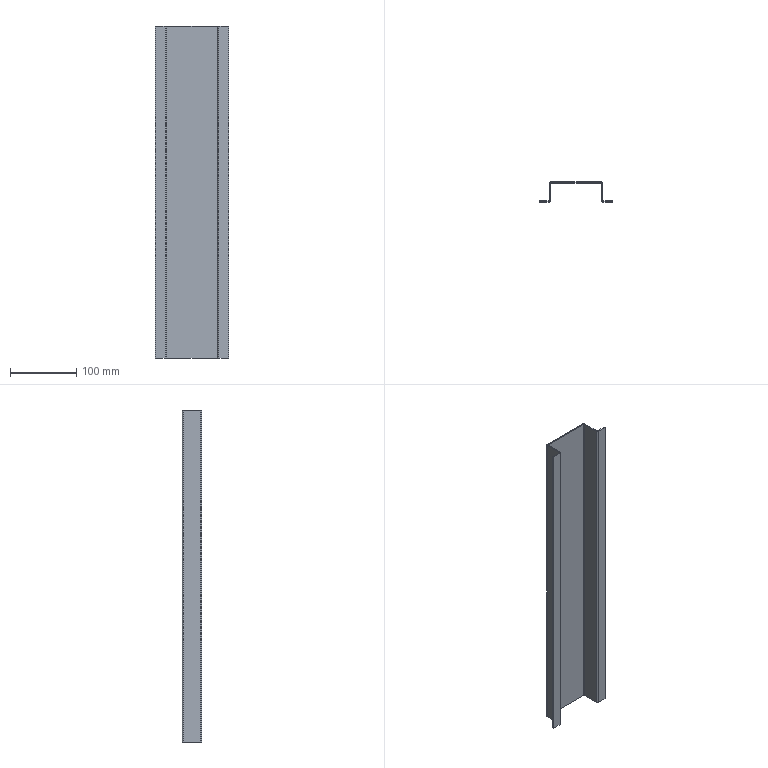Part | SolidWorks | features FlatPattern 1, SMBaseFlange 1, SheetMetal 1 | 1 solid | 38 faces | box 110 x 30 x 500 mm | volume 123640 mm3 | plane 30 | cylinder 8 | commonest cylinder face diameters 1 x4 4 x4
STEP:
#1=CARTESIAN_POINT('',(-40.,0.5,250.));
#2=VERTEX_POINT('',#1);
#3=CARTESIAN_POINT('',(-38.5,0.5,250.));
#4=VERTEX_POINT('',#3);
#5=CARTESIAN_POINT('',(-40.,0.5,250.));
#6=DIRECTION('',(1.,0.,0.));
#7=VECTOR('',#6,1000.);
#8=LINE('',#5,#7);
#9=EDGE_CURVE('',#2,#4,#8,.T.);
#10=ORIENTED_EDGE('',*,*,#9,.F.);
#11=CARTESIAN_POINT('',(-40.5,0.,250.));
#12=VERTEX_POINT('',#11);
#13=CARTESIAN_POINT('',(-40.5,0.5,250.));
#14=DIRECTION('',(0.,0.,-1.));
#15=DIRECTION('',(-1.,0.,0.));
#16=AXIS2_PLACEMENT_3D('',#13,#14,#15);
#17=CIRCLE('',#16,0.5);
#18=EDGE_CURVE('',#2,#12,#17,.T.);
#19=ORIENTED_EDGE('',*,*,#18,.T.);
#20=CARTESIAN_POINT('',(-40.5,-1.5,250.));
#21=VERTEX_POINT('',#20);
#22=CARTESIAN_POINT('',(-40.5,-1.5,250.));
#23=DIRECTION('',(0.,1.,0.));
#24=VECTOR('',#23,1000.);
#25=LINE('',#22,#24);
#26=EDGE_CURVE('',#21,#12,#25,.T.);
#27=ORIENTED_EDGE('',*,*,#26,.F.);
#28=CARTESIAN_POINT('',(-40.5,0.5,250.));
#29=DIRECTION('',(0.,0.,-1.));
#30=DIRECTION('',(1.,0.,0.));
#31=AXIS2_PLACEMENT_3D('',#28,#29,#30);
#32=CIRCLE('',#31,2.);
#33=EDGE_CURVE('',#4,#21,#32,.T.);
#34=ORIENTED_EDGE('',*,*,#33,.F.);
#35=EDGE_LOOP('',(#10,#19,#27,#34));
#36=FACE_OUTER_BOUND('',#35,.T.);
#37=CARTESIAN_POINT('',(-40.,0.5,250.));
#38=DIRECTION('',(0.,0.,1.));
#39=DIRECTION('',(1.,0.,0.));
#40=AXIS2_PLACEMENT_3D('',#37,#38,#39);
#41=PLANE('',#40);
#42=ADVANCED_FACE('',(#36),#41,.T.);
#43=CARTESIAN_POINT('',(-40.,26.5,250.));
#44=VERTEX_POINT('',#43);
#45=CARTESIAN_POINT('',(-40.,0.,250.));
#46=DIRECTION('',(0.,-1.,0.));
#47=VECTOR('',#46,1000.);
#48=LINE('',#45,#47);
#49=EDGE_CURVE('',#44,#2,#48,.T.);
#50=ORIENTED_EDGE('',*,*,#49,.T.);
#51=ORIENTED_EDGE('',*,*,#9,.T.);
#52=CARTESIAN_POINT('',(-38.5,26.5,250.));
#53=VERTEX_POINT('',#52);
#54=CARTESIAN_POINT('',(-38.5,0.,250.));
#55=DIRECTION('',(0.,-1.,0.));
#56=VECTOR('',#55,1000.);
#57=LINE('',#54,#56);
#58=EDGE_CURVE('',#53,#4,#57,.T.);
#59=ORIENTED_EDGE('',*,*,#58,.F.);
#60=CARTESIAN_POINT('',(-38.5,26.5,250.));
#61=DIRECTION('',(-1.,0.,0.));
#62=VECTOR('',#61,1000.);
#63=LINE('',#60,#62);
#64=EDGE_CURVE('',#53,#44,#63,.T.);
#65=ORIENTED_EDGE('',*,*,#64,.T.);
#66=EDGE_LOOP('',(#50,#51,#59,#65));
#67=FACE_OUTER_BOUND('',#66,.T.);
#68=CARTESIAN_POINT('',(-40.5,-1.5,250.));
#69=DIRECTION('',(0.,0.,1.));
#70=DIRECTION('',(1.,0.,0.));
#71=AXIS2_PLACEMENT_3D('',#68,#69,#70);
#72=PLANE('',#71);
#73=ADVANCED_FACE('',(#67),#72,.T.);
#74=CARTESIAN_POINT('',(-40.5,0.,-250.));
#75=VERTEX_POINT('',#74);
#76=CARTESIAN_POINT('',(-40.5,-1.5,-250.));
#77=VERTEX_POINT('',#76);
#78=CARTESIAN_POINT('',(-40.5,0.,-250.));
#79=DIRECTION('',(0.,-1.,0.));
#80=VECTOR('',#79,1000.);
#81=LINE('',#78,#80);
#82=EDGE_CURVE('',#75,#77,#81,.T.);
#83=ORIENTED_EDGE('',*,*,#82,.F.);
#84=CARTESIAN_POINT('',(-40.,0.5,-250.));
#85=VERTEX_POINT('',#84);
#86=CARTESIAN_POINT('',(-40.5,0.5,-250.));
#87=DIRECTION('',(0.,0.,-1.));
#88=DIRECTION('',(-1.,0.,0.));
#89=AXIS2_PLACEMENT_3D('',#86,#87,#88);
#90=CIRCLE('',#89,0.5);
#91=EDGE_CURVE('',#85,#75,#90,.T.);
#92=ORIENTED_EDGE('',*,*,#91,.F.);
#93=CARTESIAN_POINT('',(-38.5,0.5,-250.));
#94=VERTEX_POINT('',#93);
#95=CARTESIAN_POINT('',(-38.5,0.5,-250.));
#96=DIRECTION('',(-1.,0.,0.));
#97=VECTOR('',#96,1000.);
#98=LINE('',#95,#97);
#99=EDGE_CURVE('',#94,#85,#98,.T.);
#100=ORIENTED_EDGE('',*,*,#99,.F.);
#101=CARTESIAN_POINT('',(-40.5,0.5,-250.));
#102=DIRECTION('',(0.,0.,-1.));
#103=DIRECTION('',(1.,0.,0.));
#104=AXIS2_PLACEMENT_3D('',#101,#102,#103);
#105=CIRCLE('',#104,2.);
#106=EDGE_CURVE('',#94,#77,#105,.T.);
#107=ORIENTED_EDGE('',*,*,#106,.T.);
#108=EDGE_LOOP('',(#83,#92,#100,#107));
#109=FACE_OUTER_BOUND('',#108,.T.);
#110=CARTESIAN_POINT('',(-40.5,0.,-250.));
#111=DIRECTION('',(0.,0.,-1.));
#112=DIRECTION('',(-1.,0.,0.));
#113=AXIS2_PLACEMENT_3D('',#110,#111,#112);
#114=PLANE('',#113);
#115=ADVANCED_FACE('',(#109),#114,.T.);
#116=CARTESIAN_POINT('',(-55.,0.,-250.));
#117=VERTEX_POINT('',#116);
#118=CARTESIAN_POINT('',(-55.,0.,-250.));
#119=DIRECTION('',(-1.,0.,0.));
#120=VECTOR('',#119,1000.);
#121=LINE('',#118,#120);
#122=EDGE_CURVE('',#75,#117,#121,.T.);
#123=ORIENTED_EDGE('',*,*,#122,.F.);
#124=ORIENTED_EDGE('',*,*,#82,.T.);
#125=CARTESIAN_POINT('',(-55.,-1.5,-250.));
#126=VERTEX_POINT('',#125);
#127=CARTESIAN_POINT('',(-55.,-1.5,-250.));
#128=DIRECTION('',(-1.,0.,0.));
#129=VECTOR('',#128,1000.);
#130=LINE('',#127,#129);
#131=EDGE_CURVE('',#77,#126,#130,.T.);
#132=ORIENTED_EDGE('',*,*,#131,.T.);
#133=CARTESIAN_POINT('',(-55.,-1.5,-250.));
#134=DIRECTION('',(0.,1.,0.));
#135=VECTOR('',#134,1000.);
#136=LINE('',#133,#135);
#137=EDGE_CURVE('',#126,#117,#136,.T.);
#138=ORIENTED_EDGE('',*,*,#137,.T.);
#139=EDGE_LOOP('',(#123,#124,#132,#138));
#140=FACE_OUTER_BOUND('',#139,.T.);
#141=CARTESIAN_POINT('',(-38.5,0.5,-250.));
#142=DIRECTION('',(0.,0.,-1.));
#143=DIRECTION('',(-1.,0.,0.));
#144=AXIS2_PLACEMENT_3D('',#141,#142,#143);
#145=PLANE('',#144);
#146=ADVANCED_FACE('',(#140),#145,.T.);
#147=CARTESIAN_POINT('',(-38.,28.5,250.));
#148=VERTEX_POINT('',#147);
#149=CARTESIAN_POINT('',(-38.,27.,250.));
#150=VERTEX_POINT('',#149);
#151=CARTESIAN_POINT('',(-38.,28.5,250.));
#152=DIRECTION('',(0.,-1.,0.));
#153=VECTOR('',#152,1000.);
#154=LINE('',#151,#153);
#155=EDGE_CURVE('',#148,#150,#154,.T.);
#156=ORIENTED_EDGE('',*,*,#155,.F.);
#157=CARTESIAN_POINT('',(-38.,26.5,250.));
#158=DIRECTION('',(0.,0.,1.));
#159=DIRECTION('',(1.,0.,0.));
#160=AXIS2_PLACEMENT_3D('',#157,#158,#159);
#161=CIRCLE('',#160,2.);
#162=EDGE_CURVE('',#148,#44,#161,.T.);
#163=ORIENTED_EDGE('',*,*,#162,.T.);
#164=ORIENTED_EDGE('',*,*,#64,.F.);
#165=CARTESIAN_POINT('',(-38.,26.5,250.));
#166=DIRECTION('',(0.,0.,1.));
#167=DIRECTION('',(1.,0.,0.));
#168=AXIS2_PLACEMENT_3D('',#165,#166,#167);
#169=CIRCLE('',#168,0.5);
#170=EDGE_CURVE('',#150,#53,#169,.T.);
#171=ORIENTED_EDGE('',*,*,#170,.F.);
#172=EDGE_LOOP('',(#156,#163,#164,#171));
#173=FACE_OUTER_BOUND('',#172,.T.);
#174=CARTESIAN_POINT('',(-38.,28.5,250.));
#175=DIRECTION('',(0.,0.,1.));
#176=DIRECTION('',(1.,0.,0.));
#177=AXIS2_PLACEMENT_3D('',#174,#175,#176);
#178=PLANE('',#177);
#179=ADVANCED_FACE('',(#173),#178,.T.);
#180=CARTESIAN_POINT('',(38.,28.5,250.));
#181=VERTEX_POINT('',#180);
#182=CARTESIAN_POINT('',(-40.,28.5,250.));
#183=DIRECTION('',(-1.,0.,0.));
#184=VECTOR('',#183,1000.);
#185=LINE('',#182,#184);
#186=EDGE_CURVE('',#181,#148,#185,.T.);
#187=ORIENTED_EDGE('',*,*,#186,.T.);
#188=ORIENTED_EDGE('',*,*,#155,.T.);
#189=CARTESIAN_POINT('',(38.,27.,250.));
#190=VERTEX_POINT('',#189);
#191=CARTESIAN_POINT('',(-40.,27.,250.));
#192=DIRECTION('',(-1.,0.,0.));
#193=VECTOR('',#192,1000.);
#194=LINE('',#191,#193);
#195=EDGE_CURVE('',#190,#150,#194,.T.);
#196=ORIENTED_EDGE('',*,*,#195,.F.);
#197=CARTESIAN_POINT('',(38.,27.,250.));
#198=DIRECTION('',(0.,1.,0.));
#199=VECTOR('',#198,1000.);
#200=LINE('',#197,#199);
#201=EDGE_CURVE('',#190,#181,#200,.T.);
#202=ORIENTED_EDGE('',*,*,#201,.T.);
#203=EDGE_LOOP('',(#187,#188,#196,#202));
#204=FACE_OUTER_BOUND('',#203,.T.);
#205=CARTESIAN_POINT('',(-38.5,26.5,250.));
#206=DIRECTION('',(0.,0.,1.));
#207=DIRECTION('',(1.,0.,0.));
#208=AXIS2_PLACEMENT_3D('',#205,#206,#207);
#209=PLANE('',#208);
#210=ADVANCED_FACE('',(#204),#209,.T.);
#211=CARTESIAN_POINT('',(-40.,26.5,-250.));
#212=VERTEX_POINT('',#211);
#213=CARTESIAN_POINT('',(-38.5,26.5,-250.));
#214=VERTEX_POINT('',#213);
#215=CARTESIAN_POINT('',(-40.,26.5,-250.));
#216=DIRECTION('',(1.,0.,0.));
#217=VECTOR('',#216,1000.);
#218=LINE('',#215,#217);
#219=EDGE_CURVE('',#212,#214,#218,.T.);
#220=ORIENTED_EDGE('',*,*,#219,.F.);
#221=CARTESIAN_POINT('',(-38.,28.5,-250.));
#222=VERTEX_POINT('',#221);
#223=CARTESIAN_POINT('',(-38.,26.5,-250.));
#224=DIRECTION('',(0.,0.,1.));
#225=DIRECTION('',(1.,0.,0.));
#226=AXIS2_PLACEMENT_3D('',#223,#224,#225);
#227=CIRCLE('',#226,2.);
#228=EDGE_CURVE('',#222,#212,#227,.T.);
#229=ORIENTED_EDGE('',*,*,#228,.F.);
#230=CARTESIAN_POINT('',(-38.,27.,-250.));
#231=VERTEX_POINT('',#230);
#232=CARTESIAN_POINT('',(-38.,27.,-250.));
#233=DIRECTION('',(0.,1.,0.));
#234=VECTOR('',#233,1000.);
#235=LINE('',#232,#234);
#236=EDGE_CURVE('',#231,#222,#235,.T.);
#237=ORIENTED_EDGE('',*,*,#236,.F.);
#238=CARTESIAN_POINT('',(-38.,26.5,-250.));
#239=DIRECTION('',(0.,0.,1.));
#240=DIRECTION('',(1.,0.,0.));
#241=AXIS2_PLACEMENT_3D('',#238,#239,#240);
#242=CIRCLE('',#241,0.5);
#243=EDGE_CURVE('',#231,#214,#242,.T.);
#244=ORIENTED_EDGE('',*,*,#243,.T.);
#245=EDGE_LOOP('',(#220,#229,#237,#244));
#246=FACE_OUTER_BOUND('',#245,.T.);
#247=CARTESIAN_POINT('',(-40.,26.5,-250.));
#248=DIRECTION('',(0.,0.,-1.));
#249=DIRECTION('',(-1.,0.,0.));
#250=AXIS2_PLACEMENT_3D('',#247,#248,#249);
#251=PLANE('',#250);
#252=ADVANCED_FACE('',(#246),#251,.T.);
#253=CARTESIAN_POINT('',(-40.,0.,-250.));
#254=DIRECTION('',(0.,-1.,0.));
#255=VECTOR('',#254,1000.);
#256=LINE('',#253,#255);
#257=EDGE_CURVE('',#212,#85,#256,.T.);
#258=ORIENTED_EDGE('',*,*,#257,.F.);
#259=ORIENTED_EDGE('',*,*,#219,.T.);
#260=CARTESIAN_POINT('',(-38.5,0.,-250.));
#261=DIRECTION('',(0.,-1.,0.));
#262=VECTOR('',#261,1000.);
#263=LINE('',#260,#262);
#264=EDGE_CURVE('',#214,#94,#263,.T.);
#265=ORIENTED_EDGE('',*,*,#264,.T.);
#266=ORIENTED_EDGE('',*,*,#99,.T.);
#267=EDGE_LOOP('',(#258,#259,#265,#266));
#268=FACE_OUTER_BOUND('',#267,.T.);
#269=CARTESIAN_POINT('',(-38.,27.,-250.));
#270=DIRECTION('',(0.,0.,-1.));
#271=DIRECTION('',(-1.,0.,0.));
#272=AXIS2_PLACEMENT_3D('',#269,#270,#271);
#273=PLANE('',#272);
#274=ADVANCED_FACE('',(#268),#273,.T.);
#275=CARTESIAN_POINT('',(40.,26.5,250.));
#276=VERTEX_POINT('',#275);
#277=CARTESIAN_POINT('',(38.5,26.5,250.));
#278=VERTEX_POINT('',#277);
#279=CARTESIAN_POINT('',(40.,26.5,250.));
#280=DIRECTION('',(-1.,0.,0.));
#281=VECTOR('',#280,1000.);
#282=LINE('',#279,#281);
#283=EDGE_CURVE('',#276,#278,#282,.T.);
#284=ORIENTED_EDGE('',*,*,#283,.F.);
#285=CARTESIAN_POINT('',(38.,26.5,250.));
#286=DIRECTION('',(0.,0.,1.));
#287=DIRECTION('',(1.,0.,0.));
#288=AXIS2_PLACEMENT_3D('',#285,#286,#287);
#289=CIRCLE('',#288,2.);
#290=EDGE_CURVE('',#276,#181,#289,.T.);
#291=ORIENTED_EDGE('',*,*,#290,.T.);
#292=ORIENTED_EDGE('',*,*,#201,.F.);
#293=CARTESIAN_POINT('',(38.,26.5,250.));
#294=DIRECTION('',(0.,0.,1.));
#295=DIRECTION('',(1.,0.,0.));
#296=AXIS2_PLACEMENT_3D('',#293,#294,#295);
#297=CIRCLE('',#296,0.5);
#298=EDGE_CURVE('',#278,#190,#297,.T.);
#299=ORIENTED_EDGE('',*,*,#298,.F.);
#300=EDGE_LOOP('',(#284,#291,#292,#299));
#301=FACE_OUTER_BOUND('',#300,.T.);
#302=CARTESIAN_POINT('',(40.,26.5,250.));
#303=DIRECTION('',(0.,0.,1.));
#304=DIRECTION('',(1.,0.,0.));
#305=AXIS2_PLACEMENT_3D('',#302,#303,#304);
#306=PLANE('',#305);
#307=ADVANCED_FACE('',(#301),#306,.T.);
#308=CARTESIAN_POINT('',(40.,0.5,250.));
#309=VERTEX_POINT('',#308);
#310=CARTESIAN_POINT('',(40.,0.,250.));
#311=DIRECTION('',(0.,1.,0.));
#312=VECTOR('',#311,1000.);
#313=LINE('',#310,#312);
#314=EDGE_CURVE('',#309,#276,#313,.T.);
#315=ORIENTED_EDGE('',*,*,#314,.T.);
#316=ORIENTED_EDGE('',*,*,#283,.T.);
#317=CARTESIAN_POINT('',(38.5,0.5,250.));
#318=VERTEX_POINT('',#317);
#319=CARTESIAN_POINT('',(38.5,0.,250.));
#320=DIRECTION('',(0.,1.,0.));
#321=VECTOR('',#320,1000.);
#322=LINE('',#319,#321);
#323=EDGE_CURVE('',#318,#278,#322,.T.);
#324=ORIENTED_EDGE('',*,*,#323,.F.);
#325=CARTESIAN_POINT('',(38.5,0.5,250.));
#326=DIRECTION('',(1.,0.,0.));
#327=VECTOR('',#326,1000.);
#328=LINE('',#325,#327);
#329=EDGE_CURVE('',#318,#309,#328,.T.);
#330=ORIENTED_EDGE('',*,*,#329,.T.);
#331=EDGE_LOOP('',(#315,#316,#324,#330));
#332=FACE_OUTER_BOUND('',#331,.T.);
#333=CARTESIAN_POINT('',(38.,27.,250.));
#334=DIRECTION('',(0.,0.,1.));
#335=DIRECTION('',(1.,0.,0.));
#336=AXIS2_PLACEMENT_3D('',#333,#334,#335);
#337=PLANE('',#336);
#338=ADVANCED_FACE('',(#332),#337,.T.);
#339=CARTESIAN_POINT('',(38.,28.5,-250.));
#340=VERTEX_POINT('',#339);
#341=CARTESIAN_POINT('',(38.,27.,-250.));
#342=VERTEX_POINT('',#341);
#343=CARTESIAN_POINT('',(38.,28.5,-250.));
#344=DIRECTION('',(0.,-1.,0.));
#345=VECTOR('',#344,1000.);
#346=LINE('',#343,#345);
#347=EDGE_CURVE('',#340,#342,#346,.T.);
#348=ORIENTED_EDGE('',*,*,#347,.F.);
#349=CARTESIAN_POINT('',(40.,26.5,-250.));
#350=VERTEX_POINT('',#349);
#351=CARTESIAN_POINT('',(38.,26.5,-250.));
#352=DIRECTION('',(0.,0.,1.));
#353=DIRECTION('',(1.,0.,0.));
#354=AXIS2_PLACEMENT_3D('',#351,#352,#353);
#355=CIRCLE('',#354,2.);
#356=EDGE_CURVE('',#350,#340,#355,.T.);
#357=ORIENTED_EDGE('',*,*,#356,.F.);
#358=CARTESIAN_POINT('',(38.5,26.5,-250.));
#359=VERTEX_POINT('',#358);
#360=CARTESIAN_POINT('',(38.5,26.5,-250.));
#361=DIRECTION('',(1.,0.,0.));
#362=VECTOR('',#361,1000.);
#363=LINE('',#360,#362);
#364=EDGE_CURVE('',#359,#350,#363,.T.);
#365=ORIENTED_EDGE('',*,*,#364,.F.);
#366=CARTESIAN_POINT('',(38.,26.5,-250.));
#367=DIRECTION('',(0.,0.,1.));
#368=DIRECTION('',(1.,0.,0.));
#369=AXIS2_PLACEMENT_3D('',#366,#367,#368);
#370=CIRCLE('',#369,0.5);
#371=EDGE_CURVE('',#359,#342,#370,.T.);
#372=ORIENTED_EDGE('',*,*,#371,.T.);
#373=EDGE_LOOP('',(#348,#357,#365,#372));
#374=FACE_OUTER_BOUND('',#373,.T.);
#375=CARTESIAN_POINT('',(38.,28.5,-250.));
#376=DIRECTION('',(0.,0.,-1.));
#377=DIRECTION('',(-1.,0.,0.));
#378=AXIS2_PLACEMENT_3D('',#375,#376,#377);
#379=PLANE('',#378);
#380=ADVANCED_FACE('',(#374),#379,.T.);
#381=CARTESIAN_POINT('',(-40.,28.5,-250.));
#382=DIRECTION('',(-1.,0.,0.));
#383=VECTOR('',#382,1000.);
#384=LINE('',#381,#383);
#385=EDGE_CURVE('',#340,#222,#384,.T.);
#386=ORIENTED_EDGE('',*,*,#385,.F.);
#387=ORIENTED_EDGE('',*,*,#347,.T.);
#388=CARTESIAN_POINT('',(-40.,27.,-250.));
#389=DIRECTION('',(-1.,0.,0.));
#390=VECTOR('',#389,1000.);
#391=LINE('',#388,#390);
#392=EDGE_CURVE('',#342,#231,#391,.T.);
#393=ORIENTED_EDGE('',*,*,#392,.T.);
#394=ORIENTED_EDGE('',*,*,#236,.T.);
#395=EDGE_LOOP('',(#386,#387,#393,#394));
#396=FACE_OUTER_BOUND('',#395,.T.);
#397=CARTESIAN_POINT('',(38.5,26.5,-250.));
#398=DIRECTION('',(0.,0.,-1.));
#399=DIRECTION('',(-1.,0.,0.));
#400=AXIS2_PLACEMENT_3D('',#397,#398,#399);
#401=PLANE('',#400);
#402=ADVANCED_FACE('',(#396),#401,.T.);
#403=CARTESIAN_POINT('',(40.5,0.,250.));
#404=VERTEX_POINT('',#403);
#405=CARTESIAN_POINT('',(40.5,-1.5,250.));
#406=VERTEX_POINT('',#405);
#407=CARTESIAN_POINT('',(40.5,0.,250.));
#408=DIRECTION('',(0.,-1.,0.));
#409=VECTOR('',#408,1000.);
#410=LINE('',#407,#409);
#411=EDGE_CURVE('',#404,#406,#410,.T.);
#412=ORIENTED_EDGE('',*,*,#411,.F.);
#413=CARTESIAN_POINT('',(40.5,0.5,250.));
#414=DIRECTION('',(0.,0.,-1.));
#415=DIRECTION('',(-1.,0.,0.));
#416=AXIS2_PLACEMENT_3D('',#413,#414,#415);
#417=CIRCLE('',#416,0.5);
#418=EDGE_CURVE('',#404,#309,#417,.T.);
#419=ORIENTED_EDGE('',*,*,#418,.T.);
#420=ORIENTED_EDGE('',*,*,#329,.F.);
#421=CARTESIAN_POINT('',(40.5,0.5,250.));
#422=DIRECTION('',(0.,0.,-1.));
#423=DIRECTION('',(1.,0.,0.));
#424=AXIS2_PLACEMENT_3D('',#421,#422,#423);
#425=CIRCLE('',#424,2.);
#426=EDGE_CURVE('',#406,#318,#425,.T.);
#427=ORIENTED_EDGE('',*,*,#426,.F.);
#428=EDGE_LOOP('',(#412,#419,#420,#427));
#429=FACE_OUTER_BOUND('',#428,.T.);
#430=CARTESIAN_POINT('',(40.5,0.,250.));
#431=DIRECTION('',(0.,0.,1.));
#432=DIRECTION('',(1.,0.,0.));
#433=AXIS2_PLACEMENT_3D('',#430,#431,#432);
#434=PLANE('',#433);
#435=ADVANCED_FACE('',(#429),#434,.T.);
#436=CARTESIAN_POINT('',(55.,0.,250.));
#437=VERTEX_POINT('',#436);
#438=CARTESIAN_POINT('',(55.,0.,250.));
#439=DIRECTION('',(-1.,0.,0.));
#440=VECTOR('',#439,1000.);
#441=LINE('',#438,#440);
#442=EDGE_CURVE('',#437,#404,#441,.T.);
#443=ORIENTED_EDGE('',*,*,#442,.T.);
#444=ORIENTED_EDGE('',*,*,#411,.T.);
#445=CARTESIAN_POINT('',(55.,-1.5,250.));
#446=VERTEX_POINT('',#445);
#447=CARTESIAN_POINT('',(55.,-1.5,250.));
#448=DIRECTION('',(-1.,0.,0.));
#449=VECTOR('',#448,1000.);
#450=LINE('',#447,#449);
#451=EDGE_CURVE('',#446,#406,#450,.T.);
#452=ORIENTED_EDGE('',*,*,#451,.F.);
#453=CARTESIAN_POINT('',(55.,0.,250.));
#454=DIRECTION('',(0.,-1.,0.));
#455=VECTOR('',#454,1000.);
#456=LINE('',#453,#455);
#457=EDGE_CURVE('',#437,#446,#456,.T.);
#458=ORIENTED_EDGE('',*,*,#457,.F.);
#459=EDGE_LOOP('',(#443,#444,#452,#458));
#460=FACE_OUTER_BOUND('',#459,.T.);
#461=CARTESIAN_POINT('',(38.5,0.5,250.));
#462=DIRECTION('',(0.,0.,1.));
#463=DIRECTION('',(1.,0.,0.));
#464=AXIS2_PLACEMENT_3D('',#461,#462,#463);
#465=PLANE('',#464);
#466=ADVANCED_FACE('',(#460),#465,.T.);
#467=CARTESIAN_POINT('',(40.,0.5,-250.));
#468=VERTEX_POINT('',#467);
#469=CARTESIAN_POINT('',(38.5,0.5,-250.));
#470=VERTEX_POINT('',#469);
#471=CARTESIAN_POINT('',(40.,0.5,-250.));
#472=DIRECTION('',(-1.,0.,0.));
#473=VECTOR('',#472,1000.);
#474=LINE('',#471,#473);
#475=EDGE_CURVE('',#468,#470,#474,.T.);
#476=ORIENTED_EDGE('',*,*,#475,.F.);
#477=CARTESIAN_POINT('',(40.5,0.,-250.));
#478=VERTEX_POINT('',#477);
#479=CARTESIAN_POINT('',(40.5,0.5,-250.));
#480=DIRECTION('',(0.,0.,-1.));
#481=DIRECTION('',(-1.,0.,0.));
#482=AXIS2_PLACEMENT_3D('',#479,#480,#481);
#483=CIRCLE('',#482,0.5);
#484=EDGE_CURVE('',#478,#468,#483,.T.);
#485=ORIENTED_EDGE('',*,*,#484,.F.);
#486=CARTESIAN_POINT('',(40.5,-1.5,-250.));
#487=VERTEX_POINT('',#486);
#488=CARTESIAN_POINT('',(40.5,-1.5,-250.));
#489=DIRECTION('',(0.,1.,0.));
#490=VECTOR('',#489,1000.);
#491=LINE('',#488,#490);
#492=EDGE_CURVE('',#487,#478,#491,.T.);
#493=ORIENTED_EDGE('',*,*,#492,.F.);
#494=CARTESIAN_POINT('',(40.5,0.5,-250.));
#495=DIRECTION('',(0.,0.,-1.));
#496=DIRECTION('',(1.,0.,0.));
#497=AXIS2_PLACEMENT_3D('',#494,#495,#496);
#498=CIRCLE('',#497,2.);
#499=EDGE_CURVE('',#487,#470,#498,.T.);
#500=ORIENTED_EDGE('',*,*,#499,.T.);
#501=EDGE_LOOP('',(#476,#485,#493,#500));
#502=FACE_OUTER_BOUND('',#501,.T.);
#503=CARTESIAN_POINT('',(40.,0.5,-250.));
#504=DIRECTION('',(0.,0.,-1.));
#505=DIRECTION('',(-1.,0.,0.));
#506=AXIS2_PLACEMENT_3D('',#503,#504,#505);
#507=PLANE('',#506);
#508=ADVANCED_FACE('',(#502),#507,.T.);
#509=CARTESIAN_POINT('',(40.,0.,-250.));
#510=DIRECTION('',(0.,1.,0.));
#511=VECTOR('',#510,1000.);
#512=LINE('',#509,#511);
#513=EDGE_CURVE('',#468,#350,#512,.T.);
#514=ORIENTED_EDGE('',*,*,#513,.F.);
#515=ORIENTED_EDGE('',*,*,#475,.T.);
#516=CARTESIAN_POINT('',(38.5,0.,-250.));
#517=DIRECTION('',(0.,1.,0.));
#518=VECTOR('',#517,1000.);
#519=LINE('',#516,#518);
#520=EDGE_CURVE('',#470,#359,#519,.T.);
#521=ORIENTED_EDGE('',*,*,#520,.T.);
#522=ORIENTED_EDGE('',*,*,#364,.T.);
#523=EDGE_LOOP('',(#514,#515,#521,#522));
#524=FACE_OUTER_BOUND('',#523,.T.);
#525=CARTESIAN_POINT('',(40.5,-1.5,-250.));
#526=DIRECTION('',(0.,0.,-1.));
#527=DIRECTION('',(-1.,0.,0.));
#528=AXIS2_PLACEMENT_3D('',#525,#526,#527);
#529=PLANE('',#528);
#530=ADVANCED_FACE('',(#524),#529,.T.);
#531=ORIENTED_EDGE('',*,*,#122,.T.);
#532=CARTESIAN_POINT('',(-55.,0.,250.));
#533=VERTEX_POINT('',#532);
#534=CARTESIAN_POINT('',(-55.,0.,250.));
#535=DIRECTION('',(0.,0.,-1.));
#536=VECTOR('',#535,1000.);
#537=LINE('',#534,#536);
#538=EDGE_CURVE('',#533,#117,#537,.T.);
#539=ORIENTED_EDGE('',*,*,#538,.F.);
#540=CARTESIAN_POINT('',(-55.,0.,250.));
#541=DIRECTION('',(-1.,0.,0.));
#542=VECTOR('',#541,1000.);
#543=LINE('',#540,#542);
#544=EDGE_CURVE('',#12,#533,#543,.T.);
#545=ORIENTED_EDGE('',*,*,#544,.F.);
#546=CARTESIAN_POINT('',(-40.5,0.,250.));
#547=DIRECTION('',(0.,0.,-1.));
#548=VECTOR('',#547,1000.);
#549=LINE('',#546,#548);
#550=EDGE_CURVE('',#12,#75,#549,.T.);
#551=ORIENTED_EDGE('',*,*,#550,.T.);
#552=EDGE_LOOP('',(#531,#539,#545,#551));
#553=FACE_OUTER_BOUND('',#552,.T.);
#554=CARTESIAN_POINT('',(-55.,0.,250.));
#555=DIRECTION('',(0.,-1.,0.));
#556=DIRECTION('',(0.,0.,-1.));
#557=AXIS2_PLACEMENT_3D('',#554,#555,#556);
#558=PLANE('',#557);
#559=ADVANCED_FACE('',(#553),#558,.F.);
#560=ORIENTED_EDGE('',*,*,#137,.F.);
#561=CARTESIAN_POINT('',(-55.,-1.5,250.));
#562=VERTEX_POINT('',#561);
#563=CARTESIAN_POINT('',(-55.,-1.5,250.));
#564=DIRECTION('',(0.,0.,-1.));
#565=VECTOR('',#564,1000.);
#566=LINE('',#563,#565);
#567=EDGE_CURVE('',#562,#126,#566,.T.);
#568=ORIENTED_EDGE('',*,*,#567,.F.);
#569=CARTESIAN_POINT('',(-55.,-1.5,250.));
#570=DIRECTION('',(0.,1.,0.));
#571=VECTOR('',#570,1000.);
#572=LINE('',#569,#571);
#573=EDGE_CURVE('',#562,#533,#572,.T.);
#574=ORIENTED_EDGE('',*,*,#573,.T.);
#575=ORIENTED_EDGE('',*,*,#538,.T.);
#576=EDGE_LOOP('',(#560,#568,#574,#575));
#577=FACE_OUTER_BOUND('',#576,.T.);
#578=CARTESIAN_POINT('',(-55.,-1.5,250.));
#579=DIRECTION('',(-1.,0.,0.));
#580=DIRECTION('',(0.,0.,1.));
#581=AXIS2_PLACEMENT_3D('',#578,#579,#580);
#582=PLANE('',#581);
#583=ADVANCED_FACE('',(#577),#582,.T.);
#584=ORIENTED_EDGE('',*,*,#131,.F.);
#585=CARTESIAN_POINT('',(-40.5,-1.5,250.));
#586=DIRECTION('',(0.,0.,-1.));
#587=VECTOR('',#586,1000.);
#588=LINE('',#585,#587);
#589=EDGE_CURVE('',#21,#77,#588,.T.);
#590=ORIENTED_EDGE('',*,*,#589,.F.);
#591=CARTESIAN_POINT('',(-55.,-1.5,250.));
#592=DIRECTION('',(-1.,0.,0.));
#593=VECTOR('',#592,1000.);
#594=LINE('',#591,#593);
#595=EDGE_CURVE('',#21,#562,#594,.T.);
#596=ORIENTED_EDGE('',*,*,#595,.T.);
#597=ORIENTED_EDGE('',*,*,#567,.T.);
#598=EDGE_LOOP('',(#584,#590,#596,#597));
#599=FACE_OUTER_BOUND('',#598,.T.);
#600=CARTESIAN_POINT('',(-55.,-1.5,250.));
#601=DIRECTION('',(0.,-1.,0.));
#602=DIRECTION('',(0.,0.,-1.));
#603=AXIS2_PLACEMENT_3D('',#600,#601,#602);
#604=PLANE('',#603);
#605=ADVANCED_FACE('',(#599),#604,.T.);
#606=ORIENTED_EDGE('',*,*,#106,.F.);
#607=CARTESIAN_POINT('',(-38.5,0.5,250.));
#608=DIRECTION('',(0.,0.,-1.));
#609=VECTOR('',#608,1000.);
#610=LINE('',#607,#609);
#611=EDGE_CURVE('',#4,#94,#610,.T.);
#612=ORIENTED_EDGE('',*,*,#611,.F.);
#613=ORIENTED_EDGE('',*,*,#33,.T.);
#614=ORIENTED_EDGE('',*,*,#589,.T.);
#615=EDGE_LOOP('',(#606,#612,#613,#614));
#616=FACE_OUTER_BOUND('',#615,.T.);
#617=CARTESIAN_POINT('',(-40.5,0.5,250.));
#618=DIRECTION('',(0.,0.,-1.));
#619=DIRECTION('',(-1.,0.,0.));
#620=AXIS2_PLACEMENT_3D('',#617,#618,#619);
#621=CYLINDRICAL_SURFACE('',#620,2.);
#622=ADVANCED_FACE('',(#616),#621,.T.);
#623=ORIENTED_EDGE('',*,*,#264,.F.);
#624=CARTESIAN_POINT('',(-38.5,26.5,250.));
#625=DIRECTION('',(0.,0.,-1.));
#626=VECTOR('',#625,1000.);
#627=LINE('',#624,#626);
#628=EDGE_CURVE('',#53,#214,#627,.T.);
#629=ORIENTED_EDGE('',*,*,#628,.F.);
#630=ORIENTED_EDGE('',*,*,#58,.T.);
#631=ORIENTED_EDGE('',*,*,#611,.T.);
#632=EDGE_LOOP('',(#623,#629,#630,#631));
#633=FACE_OUTER_BOUND('',#632,.T.);
#634=CARTESIAN_POINT('',(-38.5,0.,250.));
#635=DIRECTION('',(1.,0.,0.));
#636=DIRECTION('',(0.,1.,0.));
#637=AXIS2_PLACEMENT_3D('',#634,#635,#636);
#638=PLANE('',#637);
#639=ADVANCED_FACE('',(#633),#638,.T.);
#640=ORIENTED_EDGE('',*,*,#243,.F.);
#641=CARTESIAN_POINT('',(-38.,27.,250.));
#642=DIRECTION('',(0.,0.,-1.));
#643=VECTOR('',#642,1000.);
#644=LINE('',#641,#643);
#645=EDGE_CURVE('',#150,#231,#644,.T.);
#646=ORIENTED_EDGE('',*,*,#645,.F.);
#647=ORIENTED_EDGE('',*,*,#170,.T.);
#648=ORIENTED_EDGE('',*,*,#628,.T.);
#649=EDGE_LOOP('',(#640,#646,#647,#648));
#650=FACE_OUTER_BOUND('',#649,.T.);
#651=CARTESIAN_POINT('',(-38.,26.5,250.));
#652=DIRECTION('',(0.,0.,-1.));
#653=DIRECTION('',(-1.,0.,0.));
#654=AXIS2_PLACEMENT_3D('',#651,#652,#653);
#655=CYLINDRICAL_SURFACE('',#654,0.5);
#656=ADVANCED_FACE('',(#650),#655,.F.);
#657=ORIENTED_EDGE('',*,*,#392,.F.);
#658=CARTESIAN_POINT('',(38.,27.,250.));
#659=DIRECTION('',(0.,0.,-1.));
#660=VECTOR('',#659,1000.);
#661=LINE('',#658,#660);
#662=EDGE_CURVE('',#190,#342,#661,.T.);
#663=ORIENTED_EDGE('',*,*,#662,.F.);
#664=ORIENTED_EDGE('',*,*,#195,.T.);
#665=ORIENTED_EDGE('',*,*,#645,.T.);
#666=EDGE_LOOP('',(#657,#663,#664,#665));
#667=FACE_OUTER_BOUND('',#666,.T.);
#668=CARTESIAN_POINT('',(-40.,27.,250.));
#669=DIRECTION('',(0.,-1.,0.));
#670=DIRECTION('',(0.,0.,-1.));
#671=AXIS2_PLACEMENT_3D('',#668,#669,#670);
#672=PLANE('',#671);
#673=ADVANCED_FACE('',(#667),#672,.T.);
#674=ORIENTED_EDGE('',*,*,#371,.F.);
#675=CARTESIAN_POINT('',(38.5,26.5,250.));
#676=DIRECTION('',(0.,0.,-1.));
#677=VECTOR('',#676,1000.);
#678=LINE('',#675,#677);
#679=EDGE_CURVE('',#278,#359,#678,.T.);
#680=ORIENTED_EDGE('',*,*,#679,.F.);
#681=ORIENTED_EDGE('',*,*,#298,.T.);
#682=ORIENTED_EDGE('',*,*,#662,.T.);
#683=EDGE_LOOP('',(#674,#680,#681,#682));
#684=FACE_OUTER_BOUND('',#683,.T.);
#685=CARTESIAN_POINT('',(38.,26.5,250.));
#686=DIRECTION('',(0.,0.,-1.));
#687=DIRECTION('',(-1.,0.,0.));
#688=AXIS2_PLACEMENT_3D('',#685,#686,#687);
#689=CYLINDRICAL_SURFACE('',#688,0.5);
#690=ADVANCED_FACE('',(#684),#689,.F.);
#691=ORIENTED_EDGE('',*,*,#520,.F.);
#692=CARTESIAN_POINT('',(38.5,0.5,250.));
#693=DIRECTION('',(0.,0.,-1.));
#694=VECTOR('',#693,1000.);
#695=LINE('',#692,#694);
#696=EDGE_CURVE('',#318,#470,#695,.T.);
#697=ORIENTED_EDGE('',*,*,#696,.F.);
#698=ORIENTED_EDGE('',*,*,#323,.T.);
#699=ORIENTED_EDGE('',*,*,#679,.T.);
#700=EDGE_LOOP('',(#691,#697,#698,#699));
#701=FACE_OUTER_BOUND('',#700,.T.);
#702=CARTESIAN_POINT('',(38.5,0.,250.));
#703=DIRECTION('',(-1.,0.,0.));
#704=DIRECTION('',(0.,-1.,0.));
#705=AXIS2_PLACEMENT_3D('',#702,#703,#704);
#706=PLANE('',#705);
#707=ADVANCED_FACE('',(#701),#706,.T.);
#708=ORIENTED_EDGE('',*,*,#499,.F.);
#709=CARTESIAN_POINT('',(40.5,-1.5,250.));
#710=DIRECTION('',(0.,0.,-1.));
#711=VECTOR('',#710,1000.);
#712=LINE('',#709,#711);
#713=EDGE_CURVE('',#406,#487,#712,.T.);
#714=ORIENTED_EDGE('',*,*,#713,.F.);
#715=ORIENTED_EDGE('',*,*,#426,.T.);
#716=ORIENTED_EDGE('',*,*,#696,.T.);
#717=EDGE_LOOP('',(#708,#714,#715,#716));
#718=FACE_OUTER_BOUND('',#717,.T.);
#719=CARTESIAN_POINT('',(40.5,0.5,250.));
#720=DIRECTION('',(0.,0.,-1.));
#721=DIRECTION('',(-1.,0.,0.));
#722=AXIS2_PLACEMENT_3D('',#719,#720,#721);
#723=CYLINDRICAL_SURFACE('',#722,2.);
#724=ADVANCED_FACE('',(#718),#723,.T.);
#725=CARTESIAN_POINT('',(55.,-1.5,-250.));
#726=VERTEX_POINT('',#725);
#727=CARTESIAN_POINT('',(55.,-1.5,-250.));
#728=DIRECTION('',(-1.,0.,0.));
#729=VECTOR('',#728,1000.);
#730=LINE('',#727,#729);
#731=EDGE_CURVE('',#726,#487,#730,.T.);
#732=ORIENTED_EDGE('',*,*,#731,.F.);
#733=CARTESIAN_POINT('',(55.,-1.5,250.));
#734=DIRECTION('',(0.,0.,-1.));
#735=VECTOR('',#734,1000.);
#736=LINE('',#733,#735);
#737=EDGE_CURVE('',#446,#726,#736,.T.);
#738=ORIENTED_EDGE('',*,*,#737,.F.);
#739=ORIENTED_EDGE('',*,*,#451,.T.);
#740=ORIENTED_EDGE('',*,*,#713,.T.);
#741=EDGE_LOOP('',(#732,#738,#739,#740));
#742=FACE_OUTER_BOUND('',#741,.T.);
#743=CARTESIAN_POINT('',(55.,-1.5,250.));
#744=DIRECTION('',(0.,-1.,0.));
#745=DIRECTION('',(0.,0.,-1.));
#746=AXIS2_PLACEMENT_3D('',#743,#744,#745);
#747=PLANE('',#746);
#748=ADVANCED_FACE('',(#742),#747,.T.);
#749=CARTESIAN_POINT('',(55.,0.,-250.));
#750=VERTEX_POINT('',#749);
#751=CARTESIAN_POINT('',(55.,0.,-250.));
#752=DIRECTION('',(0.,-1.,0.));
#753=VECTOR('',#752,1000.);
#754=LINE('',#751,#753);
#755=EDGE_CURVE('',#750,#726,#754,.T.);
#756=ORIENTED_EDGE('',*,*,#755,.F.);
#757=CARTESIAN_POINT('',(55.,0.,250.));
#758=DIRECTION('',(0.,0.,-1.));
#759=VECTOR('',#758,1000.);
#760=LINE('',#757,#759);
#761=EDGE_CURVE('',#437,#750,#760,.T.);
#762=ORIENTED_EDGE('',*,*,#761,.F.);
#763=ORIENTED_EDGE('',*,*,#457,.T.);
#764=ORIENTED_EDGE('',*,*,#737,.T.);
#765=EDGE_LOOP('',(#756,#762,#763,#764));
#766=FACE_OUTER_BOUND('',#765,.T.);
#767=CARTESIAN_POINT('',(55.,0.,250.));
#768=DIRECTION('',(1.,0.,0.));
#769=DIRECTION('',(0.,0.,-1.));
#770=AXIS2_PLACEMENT_3D('',#767,#768,#769);
#771=PLANE('',#770);
#772=ADVANCED_FACE('',(#766),#771,.T.);
#773=CARTESIAN_POINT('',(55.,0.,-250.));
#774=DIRECTION('',(-1.,0.,0.));
#775=VECTOR('',#774,1000.);
#776=LINE('',#773,#775);
#777=EDGE_CURVE('',#750,#478,#776,.T.);
#778=ORIENTED_EDGE('',*,*,#777,.T.);
#779=CARTESIAN_POINT('',(40.5,0.,250.));
#780=DIRECTION('',(0.,0.,-1.));
#781=VECTOR('',#780,1000.);
#782=LINE('',#779,#781);
#783=EDGE_CURVE('',#404,#478,#782,.T.);
#784=ORIENTED_EDGE('',*,*,#783,.F.);
#785=ORIENTED_EDGE('',*,*,#442,.F.);
#786=ORIENTED_EDGE('',*,*,#761,.T.);
#787=EDGE_LOOP('',(#778,#784,#785,#786));
#788=FACE_OUTER_BOUND('',#787,.T.);
#789=CARTESIAN_POINT('',(55.,0.,250.));
#790=DIRECTION('',(0.,-1.,0.));
#791=DIRECTION('',(0.,0.,-1.));
#792=AXIS2_PLACEMENT_3D('',#789,#790,#791);
#793=PLANE('',#792);
#794=ADVANCED_FACE('',(#788),#793,.F.);
#795=ORIENTED_EDGE('',*,*,#484,.T.);
#796=CARTESIAN_POINT('',(40.,0.5,250.));
#797=DIRECTION('',(0.,0.,-1.));
#798=VECTOR('',#797,1000.);
#799=LINE('',#796,#798);
#800=EDGE_CURVE('',#309,#468,#799,.T.);
#801=ORIENTED_EDGE('',*,*,#800,.F.);
#802=ORIENTED_EDGE('',*,*,#418,.F.);
#803=ORIENTED_EDGE('',*,*,#783,.T.);
#804=EDGE_LOOP('',(#795,#801,#802,#803));
#805=FACE_OUTER_BOUND('',#804,.T.);
#806=CARTESIAN_POINT('',(40.5,0.5,250.));
#807=DIRECTION('',(0.,0.,-1.));
#808=DIRECTION('',(-1.,0.,0.));
#809=AXIS2_PLACEMENT_3D('',#806,#807,#808);
#810=CYLINDRICAL_SURFACE('',#809,0.5);
#811=ADVANCED_FACE('',(#805),#810,.F.);
#812=ORIENTED_EDGE('',*,*,#513,.T.);
#813=CARTESIAN_POINT('',(40.,26.5,250.));
#814=DIRECTION('',(0.,0.,-1.));
#815=VECTOR('',#814,1000.);
#816=LINE('',#813,#815);
#817=EDGE_CURVE('',#276,#350,#816,.T.);
#818=ORIENTED_EDGE('',*,*,#817,.F.);
#819=ORIENTED_EDGE('',*,*,#314,.F.);
#820=ORIENTED_EDGE('',*,*,#800,.T.);
#821=EDGE_LOOP('',(#812,#818,#819,#820));
#822=FACE_OUTER_BOUND('',#821,.T.);
#823=CARTESIAN_POINT('',(40.,0.,250.));
#824=DIRECTION('',(-1.,0.,0.));
#825=DIRECTION('',(0.,-1.,0.));
#826=AXIS2_PLACEMENT_3D('',#823,#824,#825);
#827=PLANE('',#826);
#828=ADVANCED_FACE('',(#822),#827,.F.);
#829=ORIENTED_EDGE('',*,*,#356,.T.);
#830=CARTESIAN_POINT('',(38.,28.5,250.));
#831=DIRECTION('',(0.,0.,-1.));
#832=VECTOR('',#831,1000.);
#833=LINE('',#830,#832);
#834=EDGE_CURVE('',#181,#340,#833,.T.);
#835=ORIENTED_EDGE('',*,*,#834,.F.);
#836=ORIENTED_EDGE('',*,*,#290,.F.);
#837=ORIENTED_EDGE('',*,*,#817,.T.);
#838=EDGE_LOOP('',(#829,#835,#836,#837));
#839=FACE_OUTER_BOUND('',#838,.T.);
#840=CARTESIAN_POINT('',(38.,26.5,250.));
#841=DIRECTION('',(0.,0.,-1.));
#842=DIRECTION('',(-1.,0.,0.));
#843=AXIS2_PLACEMENT_3D('',#840,#841,#842);
#844=CYLINDRICAL_SURFACE('',#843,2.);
#845=ADVANCED_FACE('',(#839),#844,.T.);
#846=ORIENTED_EDGE('',*,*,#385,.T.);
#847=CARTESIAN_POINT('',(-38.,28.5,250.));
#848=DIRECTION('',(0.,0.,-1.));
#849=VECTOR('',#848,1000.);
#850=LINE('',#847,#849);
#851=EDGE_CURVE('',#148,#222,#850,.T.);
#852=ORIENTED_EDGE('',*,*,#851,.F.);
#853=ORIENTED_EDGE('',*,*,#186,.F.);
#854=ORIENTED_EDGE('',*,*,#834,.T.);
#855=EDGE_LOOP('',(#846,#852,#853,#854));
#856=FACE_OUTER_BOUND('',#855,.T.);
#857=CARTESIAN_POINT('',(-40.,28.5,250.));
#858=DIRECTION('',(0.,-1.,0.));
#859=DIRECTION('',(0.,0.,-1.));
#860=AXIS2_PLACEMENT_3D('',#857,#858,#859);
#861=PLANE('',#860);
#862=ADVANCED_FACE('',(#856),#861,.F.);
#863=ORIENTED_EDGE('',*,*,#228,.T.);
#864=CARTESIAN_POINT('',(-40.,26.5,250.));
#865=DIRECTION('',(0.,0.,-1.));
#866=VECTOR('',#865,1000.);
#867=LINE('',#864,#866);
#868=EDGE_CURVE('',#44,#212,#867,.T.);
#869=ORIENTED_EDGE('',*,*,#868,.F.);
#870=ORIENTED_EDGE('',*,*,#162,.F.);
#871=ORIENTED_EDGE('',*,*,#851,.T.);
#872=EDGE_LOOP('',(#863,#869,#870,#871));
#873=FACE_OUTER_BOUND('',#872,.T.);
#874=CARTESIAN_POINT('',(-38.,26.5,250.));
#875=DIRECTION('',(0.,0.,-1.));
#876=DIRECTION('',(-1.,0.,0.));
#877=AXIS2_PLACEMENT_3D('',#874,#875,#876);
#878=CYLINDRICAL_SURFACE('',#877,2.);
#879=ADVANCED_FACE('',(#873),#878,.T.);
#880=ORIENTED_EDGE('',*,*,#257,.T.);
#881=CARTESIAN_POINT('',(-40.,0.5,250.));
#882=DIRECTION('',(0.,0.,-1.));
#883=VECTOR('',#882,1000.);
#884=LINE('',#881,#883);
#885=EDGE_CURVE('',#2,#85,#884,.T.);
#886=ORIENTED_EDGE('',*,*,#885,.F.);
#887=ORIENTED_EDGE('',*,*,#49,.F.);
#888=ORIENTED_EDGE('',*,*,#868,.T.);
#889=EDGE_LOOP('',(#880,#886,#887,#888));
#890=FACE_OUTER_BOUND('',#889,.T.);
#891=CARTESIAN_POINT('',(-40.,0.,250.));
#892=DIRECTION('',(1.,0.,0.));
#893=DIRECTION('',(0.,1.,0.));
#894=AXIS2_PLACEMENT_3D('',#891,#892,#893);
#895=PLANE('',#894);
#896=ADVANCED_FACE('',(#890),#895,.F.);
#897=ORIENTED_EDGE('',*,*,#91,.T.);
#898=ORIENTED_EDGE('',*,*,#550,.F.);
#899=ORIENTED_EDGE('',*,*,#18,.F.);
#900=ORIENTED_EDGE('',*,*,#885,.T.);
#901=EDGE_LOOP('',(#897,#898,#899,#900));
#902=FACE_OUTER_BOUND('',#901,.T.);
#903=CARTESIAN_POINT('',(-40.5,0.5,250.));
#904=DIRECTION('',(0.,0.,-1.));
#905=DIRECTION('',(-1.,0.,0.));
#906=AXIS2_PLACEMENT_3D('',#903,#904,#905);
#907=CYLINDRICAL_SURFACE('',#906,0.5);
#908=ADVANCED_FACE('',(#902),#907,.F.);
#909=ORIENTED_EDGE('',*,*,#544,.T.);
#910=ORIENTED_EDGE('',*,*,#573,.F.);
#911=ORIENTED_EDGE('',*,*,#595,.F.);
#912=ORIENTED_EDGE('',*,*,#26,.T.);
#913=EDGE_LOOP('',(#909,#910,#911,#912));
#914=FACE_OUTER_BOUND('',#913,.T.);
#915=CARTESIAN_POINT('',(-40.5,0.5,250.));
#916=DIRECTION('',(0.,0.,1.));
#917=DIRECTION('',(1.,0.,0.));
#918=AXIS2_PLACEMENT_3D('',#915,#916,#917);
#919=PLANE('',#918);
#920=ADVANCED_FACE('',(#914),#919,.T.);
#921=ORIENTED_EDGE('',*,*,#731,.T.);
#922=ORIENTED_EDGE('',*,*,#492,.T.);
#923=ORIENTED_EDGE('',*,*,#777,.F.);
#924=ORIENTED_EDGE('',*,*,#755,.T.);
#925=EDGE_LOOP('',(#921,#922,#923,#924));
#926=FACE_OUTER_BOUND('',#925,.T.);
#927=CARTESIAN_POINT('',(-40.5,0.5,-250.));
#928=DIRECTION('',(0.,0.,1.));
#929=DIRECTION('',(1.,0.,0.));
#930=AXIS2_PLACEMENT_3D('',#927,#928,#929);
#931=PLANE('',#930);
#932=ADVANCED_FACE('',(#926),#931,.F.);
#933=CLOSED_SHELL('',(#42,#73,#115,#146,#179,#210,#252,#274,#307,#338,#380,#402,#435,#466,#508,#530,#559,#583,#605,#622,#639,#656,#673,#690,#707,#724,#748,#772,#794,#811,#828,#845,#862,#879,#896,#908,#920,#932));
#934=MANIFOLD_SOLID_BREP('',#933);
#935=CARTESIAN_POINT('',(0.,0.,0.));
#936=DIRECTION('',(0.,0.,1.));
#937=DIRECTION('',(1.,0.,0.));
#938=AXIS2_PLACEMENT_3D('',#935,#936,#937);
#939=(LENGTH_UNIT()NAMED_UNIT(*)SI_UNIT(.MILLI.,.METRE.));
#940=UNCERTAINTY_MEASURE_WITH_UNIT(LENGTH_MEASURE(0.00001),#939,'','');
#941=(NAMED_UNIT(*)PLANE_ANGLE_UNIT()SI_UNIT($,.RADIAN.));
#942=(NAMED_UNIT(*)SI_UNIT($,.STERADIAN.)SOLID_ANGLE_UNIT());
#943=(GEOMETRIC_REPRESENTATION_CONTEXT(3)GLOBAL_UNCERTAINTY_ASSIGNED_CONTEXT((#940))GLOBAL_UNIT_ASSIGNED_CONTEXT((#939,#941,#942))REPRESENTATION_CONTEXT('',''));
#944=ADVANCED_BREP_SHAPE_REPRESENTATION('',(#934,#938),#943);